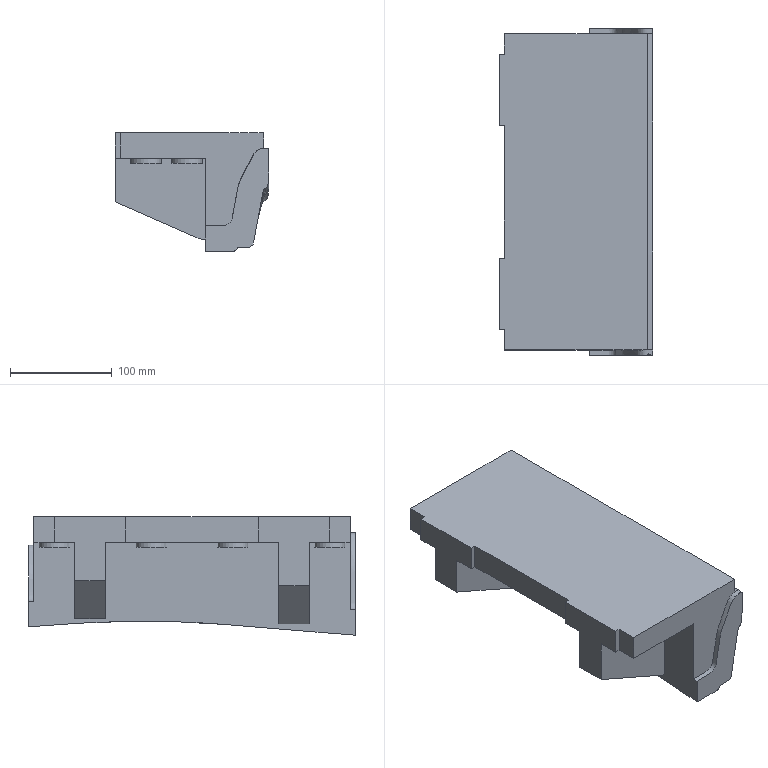Part | NX | features solid 2 | 1 solid | 79 faces | box 150.317 x 320 x 116.162 mm | volume 2862759 mm3 | spline 44 | plane 27 | cylinder 8 | commonest cylinder face diameters 30 x6 6.001 x2